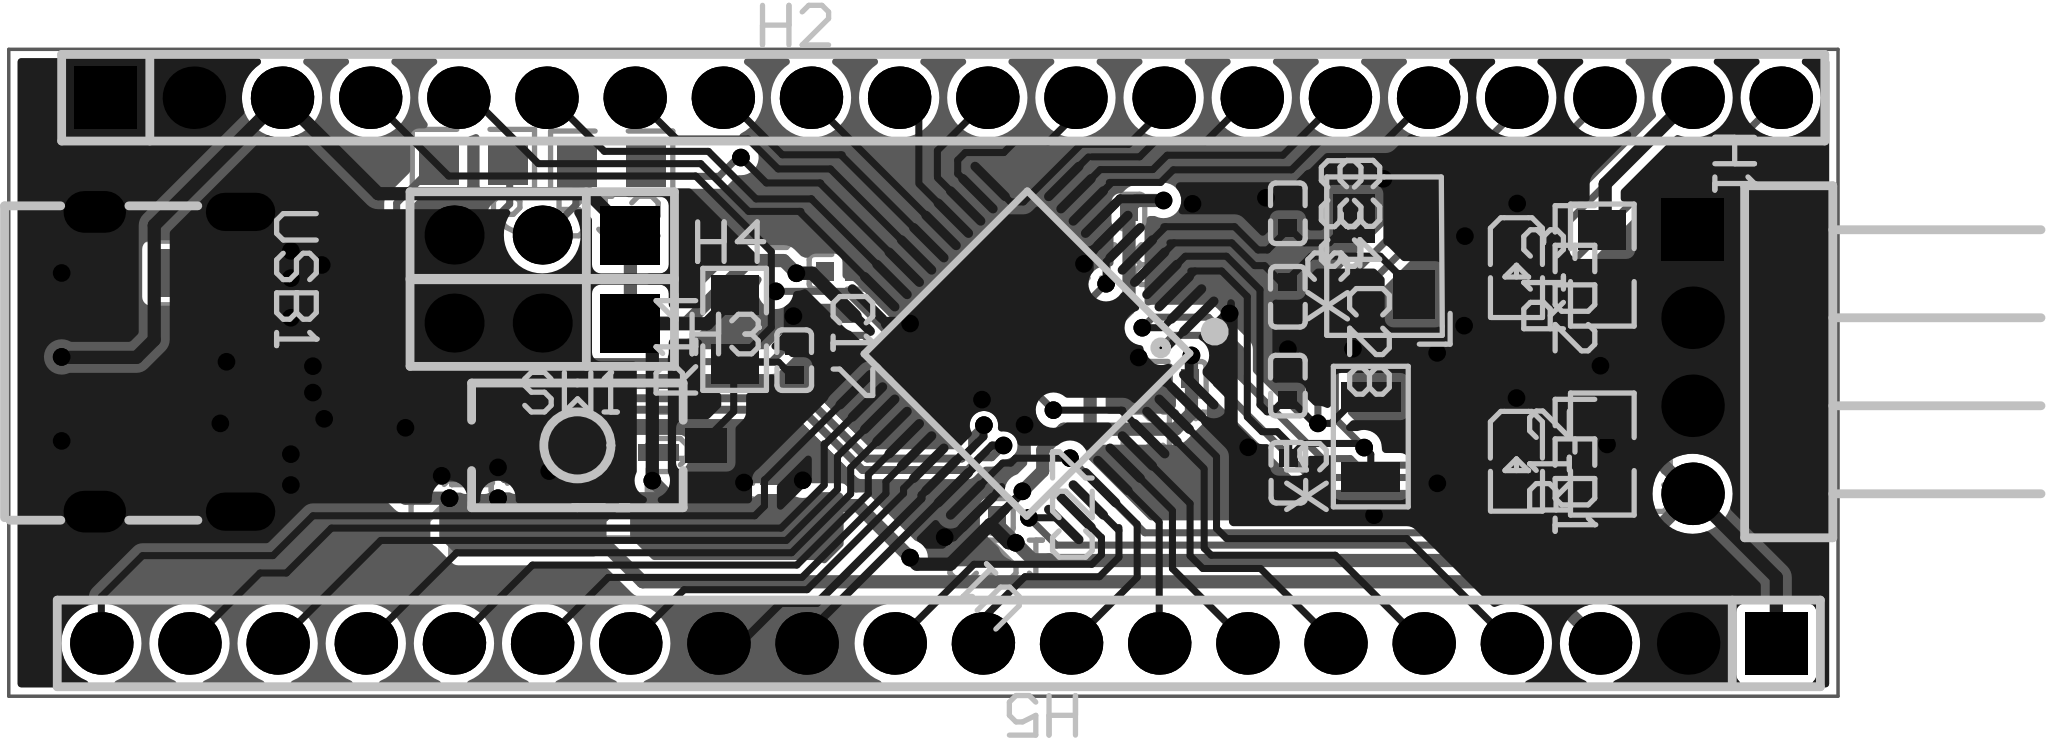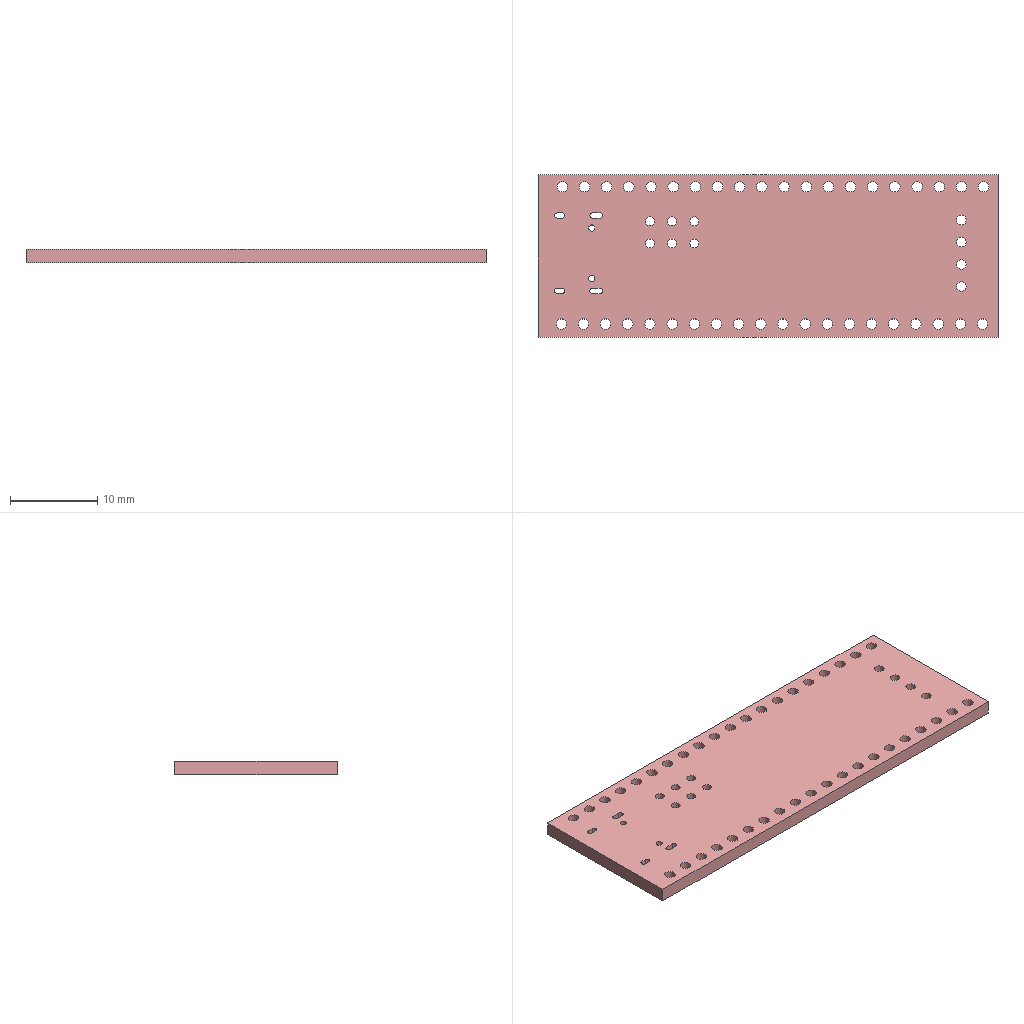Circuit board layout | Altium Designer | box 52.7 x 18.7 x 1.6 mm
Layer stack:
# Altium Designer layer stack of  (unit mm; dielectric type: 0 none, 1 core, 2 prepreg, 3 surface material)
index,name,kind,layer,copper_thickness_mm,dielectric_type,dielectric_thickness_mm,dielectric_material,dielectric_constant
0,Top Paste Mask Layer,other,,,,,,
1,Top Silkscreen Layer,other,,,,,,
2,Top Solder Mask Layer,dielectric,,,3,0.01,,3.3
3,Top Layer,copper,Top Layer,0.035,,,,
4,Dielectric1,dielectric,,,3,1.51,FR4,4.5
5,Bottom Layer,copper,Bottom Layer,0.035,,,,
6,Bottom Solder Mask Layer,dielectric,,,3,0.01,,3.3
7,Bottom Silkscreen Layer,other,,,,,,
8,Bottom Paste Mask Layer,other,,,,,,
# drill layer pairs: low layer,high layer
drill_pair,Top Layer,Bottom Layer
Part placement:
Designator,Comment,Layer,Footprint,Center-X(mm),Center-Y(mm),Rotation
U1,STM32F103C8T6,TopLayer,LQFP-48_L7.0-W7.0-P0.50-LS9.0-BL,113.206,99.619,135
R9,5.1kΩ,BottomLayer,R0805,87.536,97.081,180
R10,5.1kΩ,BottomLayer,R0805,87.536,101.927,180
C33,12pF,TopLayer,C0402,120.722,103.65,270
C15,100nF,BottomLayer,C0402,98.734,95.634,270
LDO1,ME6211C33M5G-N,BottomLayer,SOT-23-5_L3.0-W1.7-P0.95-LS2.8-BL,101.443,95.809,90
C24,1uF,BottomLayer,C0402,104.373,95.634,270
SW1,TS-1101-B-W,TopLayer,KEY-SMD_2P-L6.0-W3.6-P7.4-LS8.0-L,100.252,96.952,0
R16,10kΩ,BottomLayer,R0805,97.257,105.154,0
R15,10kΩ,BottomLayer,R0805,101.241,105.106,0
H3,PZ254V-11-03P,TopLayer,HDR-TH_3P-P2.54-V-M_PZ254V-11-03P,99.24,100.482,180
H4,PZ254V-11-03P,TopLayer,HDR-TH_3P-P2.54-V-M_PZ254V-11-03P,99.24,103.022,180
C18,100nF,BottomLayer,C0402,115.726,103.701,0
C19,100nF,BottomLayer,C0402,117.494,98.875,0
C20,100nF,BottomLayer,C0402,107.805,101.961,180
C21,100nF,BottomLayer,C0402,111.936,94.92,0
C23,1uF,BottomLayer,C0402,97.306,95.634,270
H1,DZ254W-11-04-65,TopLayer,HDR-TH_4P-P2.54-H-M-W10.3,132.383,99.365,270
C22,100nF,BottomLayer,C0402,129.903,96.129,90
H2,2.54-1*20P直针,TopLayer,HDR-TH_20P-P2.54-V-M-1,110.793,106.985,0
H5,2.54-1*20P直针,TopLayer,HDR-TH_20P-P2.54-V-M-1,110.666,91.237,180
C34,12pF,TopLayer,C0402,120.722,101.24,270
R11,1.5kΩ,BottomLayer,R0805,87.536,99.504,180
C16,100nF,BottomLayer,C0402,105.801,95.634,270
R12,1kΩ,TopLayer,R0805,129.783,96.701,90
R13,1kΩ,TopLayer,R0805,129.783,102.155,90
LED1,NCD0603R1,TopLayer,LED0603-RD_RED,127.303,96.444,270
LED2,NCD0603B1,TopLayer,LED0603-RD,127.303,102.032,270
R14,10kΩ,TopLayer,R0805,104.783,100.3,90
C17,100nF,TopLayer,C0402,106.5,99.411,270
C28,12pF,TopLayer,C0402,120.723,98.677,270
USB1,TYPE-C 16PIN 2MD(073),TopLayer,USB-C-SMD_TYPE-C-6PIN-2MD-073,88.723,99.365,270
C27,12pF,TopLayer,C0402,120.737,96.162,90
X3,8MHz,TopLayer,CRYSTAL-SMD_4P-L3.2-W2.5-BL-1,123.493,102.413,90
X5,32.768kHz,TopLayer,OSC-SMD_L3.2-W1.5,123.112,97.206,90
Pad and via stacks:
# Altium Designer via and pad stacks of  (unit mm). Each distinct definition once, with the count of objects using it.
# via: kind,start_layer,end_layer,hole_mm,diameter_mm,mode(0 simple;1 top-mid-bottom;2 full stack),diameter_per_layer,count,example_net
# pad: kind,layer,hole_mm,hole_type(0 round;1 square;2 slot),plating,top_size,top_shape(1 round;2 rect;3 octagon;9 rounded rect),mid_size,bottom_size,mode,footprint,size_per_layer,count,example
pad,Top Layer,0,0,plated,0.27x1.5,1,0.27x1.5,0.27x1.5,0,LQFP-48_L7.0-W7.0-P0.50-LS9.0-BL,,24,U1.1
pad,Top Layer,0,0,plated,1.5x0.27,1,1.5x0.27,1.5x0.27,0,LQFP-48_L7.0-W7.0-P0.50-LS9.0-BL,,24,U1.13
pad,Top Layer,0,0,plated,0.5x0.54,2,0.5x0.54,0.5x0.54,0,C0402,,10,C33.2
pad,Top Layer,0,0,plated,1.2x1,2,1.2x1,1.2x1,0,KEY-SMD_2P-L6.0-W3.6-P7.4-LS8.0-L,,2,SW1.1
pad,Top Layer,0,0,plated,1.133x1.377,2,1.133x1.377,1.133x1.377,0,R0805,,6,R12.2
pad,Top Layer,0,0,plated,0.8x0.8,2,0.8x0.8,0.8x0.8,0,LED0603-RD_RED,,2,LED1.1
pad,Top Layer,0,0,plated,0.8x0.8,2,0.8x0.8,0.8x0.8,0,LED0603-RD,,2,LED2.2
pad,Top Layer,0,0,plated,0.55x1.1,2,0.55x1.1,0.55x1.1,0,USB-C-SMD_TYPE-C-6PIN-2MD-073,,4,USB1.1
pad,Top Layer,0,0,plated,0.3x1.1,2,0.3x1.1,0.3x1.1,0,USB-C-SMD_TYPE-C-6PIN-2MD-073,,8,USB1.3
pad,Top Layer,0,0,plated,1.4x1.2,2,1.4x1.2,1.4x1.2,0,CRYSTAL-SMD_4P-L3.2-W2.5-BL-1,,4,X3.1
pad,Top Layer,0,0,plated,0.85x1.7,2,0.85x1.7,0.85x1.7,0,OSC-SMD_L3.2-W1.5,,2,X5.1
pad,Bottom Layer,0,0,plated,1.133x1.377,2,1.133x1.377,1.133x1.377,0,R0805,,10,R9.2
pad,Bottom Layer,0,0,plated,0.5x0.54,2,0.5x0.54,0.5x0.54,0,C0402,,18,C15.2
pad,Bottom Layer,0,0,plated,0.49x1.157,2,0.49x1.157,0.49x1.157,0,SOT-23-5_L3.0-W1.7-P0.95-LS2.8-BL,,3,LDO1.1
pad,Bottom Layer,0,0,plated,0.49x1.175,2,0.49x1.175,0.49x1.175,0,SOT-23-5_L3.0-W1.7-P0.95-LS2.8-BL,,2,LDO1.4
pad,Multi-Layer,1.02,0,plated,1.7x1.7,2,1.7x1.7,1.7x1.7,0,HDR-TH_3P-P2.54-V-M_PZ254V-11-03P,,2,H3.1
pad,Multi-Layer,1.02,0,plated,1.7x1.7,1,1.7x1.7,1.7x1.7,0,HDR-TH_3P-P2.54-V-M_PZ254V-11-03P,,4,H3.2
pad,Multi-Layer,1.1,0,plated,1.8x1.8,1,1.8x1.8,1.8x1.8,0,HDR-TH_4P-P2.54-H-M-W10.3,,3,H1.4
pad,Multi-Layer,1.1,0,plated,1.8x1.8,2,1.8x1.8,1.8x1.8,0,HDR-TH_4P-P2.54-H-M-W10.3,,1,H1.1
pad,Multi-Layer,1.2,0,plated,1.8x1.8,1,1.8x1.8,1.8x1.8,0,HDR-TH_20P-P2.54-V-M-1,,38,H2.20
pad,Multi-Layer,1.2,0,plated,1.8x1.8,2,1.8x1.8,1.8x1.8,0,HDR-TH_20P-P2.54-V-M-1,,2,H2.1
pad,Multi-Layer,0.6,2,plated,1.1x2,1,1.1x2,1.1x2,0,USB-C-SMD_TYPE-C-6PIN-2MD-073,,2,USB1.13
pad,Multi-Layer,0.6,2,plated,1.2x1.8,1,1.2x1.8,1.2x1.8,0,USB-C-SMD_TYPE-C-6PIN-2MD-073,,2,USB1.13
via,Top Layer,Bottom Layer,0.3048,0.508,0,,64,GND
Copper pours:
name,layer,net,type(0 solid;1 hatched;2 none)
Bottom Layer-+5V,Bottom Layer,+5V,0
Bottom Layer-3V3,Bottom Layer,3V3,0
Bottom Layer-3V3 1,Bottom Layer,3V3,0
Bottom Layer-GND,Bottom Layer,GND,0
Top Layer-GND,Top Layer,GND,0
Design rules, without the lines most boards share:
# Altium Designer design rules of  (exported by Altium Designer, unit mm)
# columns: name | kind | enabled | priority | scope1 | scope2 | descriptor | typed fields (field=value)
safeClearance1 | 0 | enabled | 2 | (InNet('USB_D-_PA11')) | (InNet('GND')) | Clearance Constraint (Gap=6mil) ((InNet('USB_D-_PA11'))),((InNet('GND'))) | gap=0.1524
safeClearance1_1 | 63 | enabled | 2 | All | All | Board Clearance Constraint (Gap=0mil) (All) |
copperThickness1oz | 0 | enabled | 3 | All | All | Clearance Constraint (Gap=5.984mil) (All),(All) | gap=0.152
copperThickness1oz_1 | 63 | enabled | 3 | All | All | Board Clearance Constraint (Gap=0mil) (All) |
pwr | 2 | enabled | 1 | (InNet('+5V') OR InNet('GND') OR InNet('3V3')) | All | Width Constraint (Min=5mil) (Max=100mil) (Preferred=15mil) ((InNet('+5V') OR InNet('GND') OR InNet('3V3'))) |
copperThickness1oz_2 | 2 | enabled | 2 | All | All | Width Constraint (Min=5mil) (Max=100mil) (Preferred=8mil) (All) |
differentialPair | 51 | enabled | 1 | All | All | Differential Pairs Uncoupled Length using the Gap Constraints (Min=4mil) (Max=5mil) (Prefered=5mil)  and Width Constraints (Min=5mil) (Max=100mil) (Prefered=9mil) (All) |
viaSize | 11 | enabled | 1 | All | All | Routing Via (MinHoleWidth=11.811mil) (MaxHoleWidth=248.031mil) (PreferredHoleWidth=12mil) (MinWidth=19.685mil) (MaxWidth=393.701mil) (PreferedWidth=20mil) (All) | via_min_hole=0.3 via_max_hole=6.3 via_preferred_diameter=0.508 via_preferred_hole=0.3048
copperRegion_Top Layer | 20 | enabled | 1 | (InNet('GND')) And OnLayer('Top Layer') | All | Polygon Connect Rule(Direct Connect )(Conductor Width=10mil) (Relief Angle=90 Angle) (Entries=4) (Air Gap Width=10mil) ((InNet('GND')) And OnLayer('Top Layer')),(All) | connect_style(0=relief,1=direct,2=none)=1 relief_conductor_width=0.254 relief_entries=4
copperRegion_Bottom Layer | 20 | enabled | 2 | (InNet('GND')) And OnLayer('Bottom Layer') | All | Polygon Connect Rule(Direct Connect )(Conductor Width=10mil) (Relief Angle=90 Angle) (Entries=4) (Air Gap Width=10mil) ((InNet('GND')) And OnLayer('Bottom Layer')),(All) | connect_style(0=relief,1=direct,2=none)=1 relief_conductor_width=0.254 relief_entries=4
copperRegion | 20 | enabled | 3 | (InNet('GND')) | All | Polygon Connect Rule(Direct Connect )(Conductor Width=10mil) (Relief Angle=90 Angle) (Entries=4) (Air Gap Width=10mil) ((InNet('GND'))),(All) | connect_style(0=relief,1=direct,2=none)=1 relief_conductor_width=0.254 relief_entries=4